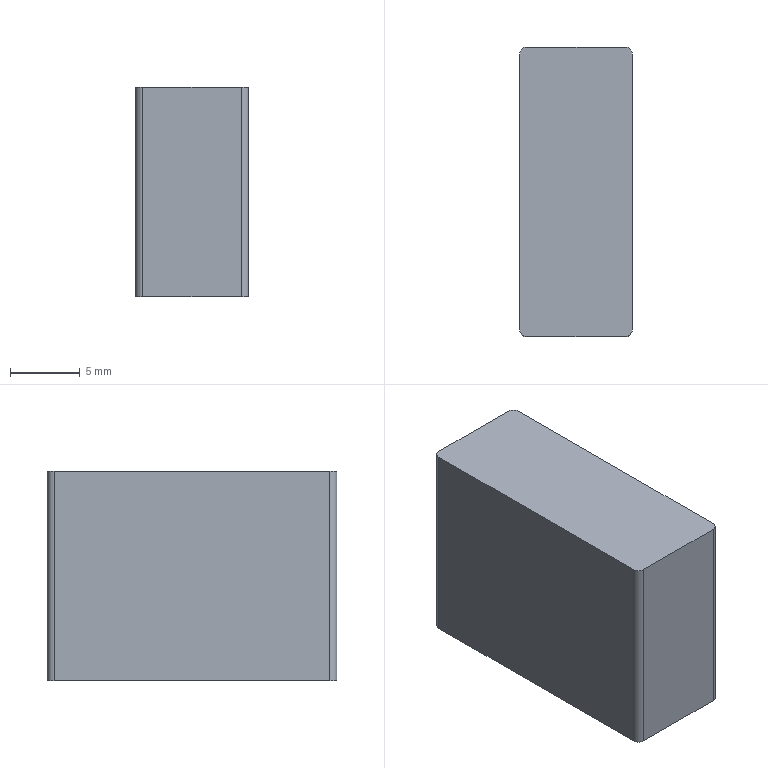Part | NX | features BREP 1 | 1 solid | 10 faces | box 8.05 x 20.702 x 15 mm | volume 2497 mm3 | plane 6 | cylinder 4 | commonest cylinder face diameters 1 x4
STEP:
#1=CARTESIAN_POINT('',(-3.525,10.351,-25.6));
#2=VERTEX_POINT('',#1);
#3=CARTESIAN_POINT('',(-4.025,9.851,-25.6));
#4=VERTEX_POINT('',#3);
#5=CARTESIAN_POINT('',(-3.525,9.851,-25.6));
#6=DIRECTION('',(0.,0.,1.));
#7=DIRECTION('',(1.,0.,0.));
#8=AXIS2_PLACEMENT_3D('',#5,#6,#7);
#9=CIRCLE('',#8,0.5);
#10=EDGE_CURVE('',#2,#4,#9,.T.);
#11=ORIENTED_EDGE('',*,*,#10,.F.);
#12=CARTESIAN_POINT('',(-3.525,10.351,-40.6));
#13=VERTEX_POINT('',#12);
#14=CARTESIAN_POINT('',(-3.525,10.351,-40.6));
#15=DIRECTION('',(0.,0.,1.));
#16=VECTOR('',#15,1000.);
#17=LINE('',#14,#16);
#18=EDGE_CURVE('',#13,#2,#17,.T.);
#19=ORIENTED_EDGE('',*,*,#18,.F.);
#20=CARTESIAN_POINT('',(-4.025,9.851,-40.6));
#21=VERTEX_POINT('',#20);
#22=CARTESIAN_POINT('',(-3.525,9.851,-40.6));
#23=DIRECTION('',(0.,0.,1.));
#24=DIRECTION('',(1.,0.,0.));
#25=AXIS2_PLACEMENT_3D('',#22,#23,#24);
#26=CIRCLE('',#25,0.5);
#27=EDGE_CURVE('',#13,#21,#26,.T.);
#28=ORIENTED_EDGE('',*,*,#27,.T.);
#29=CARTESIAN_POINT('',(-4.025,9.851,-40.6));
#30=DIRECTION('',(0.,0.,1.));
#31=VECTOR('',#30,1000.);
#32=LINE('',#29,#31);
#33=EDGE_CURVE('',#21,#4,#32,.T.);
#34=ORIENTED_EDGE('',*,*,#33,.T.);
#35=EDGE_LOOP('',(#11,#19,#28,#34));
#36=FACE_BOUND('',#35,.T.);
#37=CARTESIAN_POINT('',(-3.525,9.851,-40.6));
#38=DIRECTION('',(0.,0.,1.));
#39=DIRECTION('',(-1.,0.,0.));
#40=AXIS2_PLACEMENT_3D('',#37,#38,#39);
#41=CYLINDRICAL_SURFACE('',#40,0.5);
#42=ADVANCED_FACE('',(#36),#41,.T.);
#43=CARTESIAN_POINT('',(-4.025,-9.851,-25.6));
#44=VERTEX_POINT('',#43);
#45=CARTESIAN_POINT('',(-4.025,-9.851,-25.6));
#46=DIRECTION('',(0.,1.,0.));
#47=VECTOR('',#46,1000.);
#48=LINE('',#45,#47);
#49=EDGE_CURVE('',#44,#4,#48,.T.);
#50=ORIENTED_EDGE('',*,*,#49,.T.);
#51=ORIENTED_EDGE('',*,*,#33,.F.);
#52=CARTESIAN_POINT('',(-4.025,-9.851,-40.6));
#53=VERTEX_POINT('',#52);
#54=CARTESIAN_POINT('',(-4.025,-9.851,-40.6));
#55=DIRECTION('',(0.,1.,0.));
#56=VECTOR('',#55,1000.);
#57=LINE('',#54,#56);
#58=EDGE_CURVE('',#53,#21,#57,.T.);
#59=ORIENTED_EDGE('',*,*,#58,.F.);
#60=CARTESIAN_POINT('',(-4.025,-9.851,-40.6));
#61=DIRECTION('',(0.,0.,1.));
#62=VECTOR('',#61,1000.);
#63=LINE('',#60,#62);
#64=EDGE_CURVE('',#53,#44,#63,.T.);
#65=ORIENTED_EDGE('',*,*,#64,.T.);
#66=EDGE_LOOP('',(#50,#51,#59,#65));
#67=FACE_BOUND('',#66,.T.);
#68=CARTESIAN_POINT('',(-4.025,-9.851,-40.6));
#69=DIRECTION('',(1.,0.,0.));
#70=DIRECTION('',(0.,0.,1.));
#71=AXIS2_PLACEMENT_3D('',#68,#69,#70);
#72=PLANE('',#71);
#73=ADVANCED_FACE('',(#67),#72,.F.);
#74=CARTESIAN_POINT('',(-3.525,-10.351,-25.6));
#75=VERTEX_POINT('',#74);
#76=CARTESIAN_POINT('',(-3.525,-9.851,-25.6));
#77=DIRECTION('',(0.,0.,1.));
#78=DIRECTION('',(1.,0.,0.));
#79=AXIS2_PLACEMENT_3D('',#76,#77,#78);
#80=CIRCLE('',#79,0.5);
#81=EDGE_CURVE('',#44,#75,#80,.T.);
#82=ORIENTED_EDGE('',*,*,#81,.F.);
#83=ORIENTED_EDGE('',*,*,#64,.F.);
#84=CARTESIAN_POINT('',(-3.525,-10.351,-40.6));
#85=VERTEX_POINT('',#84);
#86=CARTESIAN_POINT('',(-3.525,-9.851,-40.6));
#87=DIRECTION('',(0.,0.,1.));
#88=DIRECTION('',(1.,0.,0.));
#89=AXIS2_PLACEMENT_3D('',#86,#87,#88);
#90=CIRCLE('',#89,0.5);
#91=EDGE_CURVE('',#53,#85,#90,.T.);
#92=ORIENTED_EDGE('',*,*,#91,.T.);
#93=CARTESIAN_POINT('',(-3.525,-10.351,-40.6));
#94=DIRECTION('',(0.,0.,1.));
#95=VECTOR('',#94,1000.);
#96=LINE('',#93,#95);
#97=EDGE_CURVE('',#85,#75,#96,.T.);
#98=ORIENTED_EDGE('',*,*,#97,.T.);
#99=EDGE_LOOP('',(#82,#83,#92,#98));
#100=FACE_BOUND('',#99,.T.);
#101=CARTESIAN_POINT('',(-3.525,-9.851,-40.6));
#102=DIRECTION('',(0.,0.,1.));
#103=DIRECTION('',(-1.,0.,0.));
#104=AXIS2_PLACEMENT_3D('',#101,#102,#103);
#105=CYLINDRICAL_SURFACE('',#104,0.5);
#106=ADVANCED_FACE('',(#100),#105,.T.);
#107=CARTESIAN_POINT('',(3.525,-10.351,-25.6));
#108=VERTEX_POINT('',#107);
#109=CARTESIAN_POINT('',(3.525,-10.351,-25.6));
#110=DIRECTION('',(-1.,0.,0.));
#111=VECTOR('',#110,1000.);
#112=LINE('',#109,#111);
#113=EDGE_CURVE('',#108,#75,#112,.T.);
#114=ORIENTED_EDGE('',*,*,#113,.T.);
#115=ORIENTED_EDGE('',*,*,#97,.F.);
#116=CARTESIAN_POINT('',(3.525,-10.351,-40.6));
#117=VERTEX_POINT('',#116);
#118=CARTESIAN_POINT('',(3.525,-10.351,-40.6));
#119=DIRECTION('',(-1.,0.,0.));
#120=VECTOR('',#119,1000.);
#121=LINE('',#118,#120);
#122=EDGE_CURVE('',#117,#85,#121,.T.);
#123=ORIENTED_EDGE('',*,*,#122,.F.);
#124=CARTESIAN_POINT('',(3.525,-10.351,-40.6));
#125=DIRECTION('',(0.,0.,1.));
#126=VECTOR('',#125,1000.);
#127=LINE('',#124,#126);
#128=EDGE_CURVE('',#117,#108,#127,.T.);
#129=ORIENTED_EDGE('',*,*,#128,.T.);
#130=EDGE_LOOP('',(#114,#115,#123,#129));
#131=FACE_BOUND('',#130,.T.);
#132=CARTESIAN_POINT('',(3.525,-10.351,-40.6));
#133=DIRECTION('',(0.,1.,0.));
#134=DIRECTION('',(0.,0.,-1.));
#135=AXIS2_PLACEMENT_3D('',#132,#133,#134);
#136=PLANE('',#135);
#137=ADVANCED_FACE('',(#131),#136,.F.);
#138=CARTESIAN_POINT('',(4.025,-9.851,-25.6));
#139=VERTEX_POINT('',#138);
#140=CARTESIAN_POINT('',(3.525,-9.851,-25.6));
#141=DIRECTION('',(0.,0.,1.));
#142=DIRECTION('',(1.,0.,0.));
#143=AXIS2_PLACEMENT_3D('',#140,#141,#142);
#144=CIRCLE('',#143,0.5);
#145=EDGE_CURVE('',#108,#139,#144,.T.);
#146=ORIENTED_EDGE('',*,*,#145,.F.);
#147=ORIENTED_EDGE('',*,*,#128,.F.);
#148=CARTESIAN_POINT('',(4.025,-9.851,-40.6));
#149=VERTEX_POINT('',#148);
#150=CARTESIAN_POINT('',(3.525,-9.851,-40.6));
#151=DIRECTION('',(0.,0.,1.));
#152=DIRECTION('',(1.,0.,0.));
#153=AXIS2_PLACEMENT_3D('',#150,#151,#152);
#154=CIRCLE('',#153,0.5);
#155=EDGE_CURVE('',#117,#149,#154,.T.);
#156=ORIENTED_EDGE('',*,*,#155,.T.);
#157=CARTESIAN_POINT('',(4.025,-9.851,-40.6));
#158=DIRECTION('',(0.,0.,1.));
#159=VECTOR('',#158,1000.);
#160=LINE('',#157,#159);
#161=EDGE_CURVE('',#149,#139,#160,.T.);
#162=ORIENTED_EDGE('',*,*,#161,.T.);
#163=EDGE_LOOP('',(#146,#147,#156,#162));
#164=FACE_BOUND('',#163,.T.);
#165=CARTESIAN_POINT('',(3.525,-9.851,-40.6));
#166=DIRECTION('',(0.,0.,1.));
#167=DIRECTION('',(-1.,0.,0.));
#168=AXIS2_PLACEMENT_3D('',#165,#166,#167);
#169=CYLINDRICAL_SURFACE('',#168,0.5);
#170=ADVANCED_FACE('',(#164),#169,.T.);
#171=CARTESIAN_POINT('',(4.025,9.851,-25.6));
#172=VERTEX_POINT('',#171);
#173=CARTESIAN_POINT('',(4.025,9.851,-25.6));
#174=DIRECTION('',(0.,-1.,0.));
#175=VECTOR('',#174,1000.);
#176=LINE('',#173,#175);
#177=EDGE_CURVE('',#172,#139,#176,.T.);
#178=ORIENTED_EDGE('',*,*,#177,.T.);
#179=ORIENTED_EDGE('',*,*,#161,.F.);
#180=CARTESIAN_POINT('',(4.025,9.851,-40.6));
#181=VERTEX_POINT('',#180);
#182=CARTESIAN_POINT('',(4.025,9.851,-40.6));
#183=DIRECTION('',(0.,-1.,0.));
#184=VECTOR('',#183,1000.);
#185=LINE('',#182,#184);
#186=EDGE_CURVE('',#181,#149,#185,.T.);
#187=ORIENTED_EDGE('',*,*,#186,.F.);
#188=CARTESIAN_POINT('',(4.025,9.851,-40.6));
#189=DIRECTION('',(0.,0.,1.));
#190=VECTOR('',#189,1000.);
#191=LINE('',#188,#190);
#192=EDGE_CURVE('',#181,#172,#191,.T.);
#193=ORIENTED_EDGE('',*,*,#192,.T.);
#194=EDGE_LOOP('',(#178,#179,#187,#193));
#195=FACE_BOUND('',#194,.T.);
#196=CARTESIAN_POINT('',(4.025,9.851,-40.6));
#197=DIRECTION('',(-1.,0.,0.));
#198=DIRECTION('',(0.,1.,0.));
#199=AXIS2_PLACEMENT_3D('',#196,#197,#198);
#200=PLANE('',#199);
#201=ADVANCED_FACE('',(#195),#200,.F.);
#202=CARTESIAN_POINT('',(3.525,10.351,-25.6));
#203=VERTEX_POINT('',#202);
#204=CARTESIAN_POINT('',(3.525,9.851,-25.6));
#205=DIRECTION('',(0.,0.,1.));
#206=DIRECTION('',(1.,0.,0.));
#207=AXIS2_PLACEMENT_3D('',#204,#205,#206);
#208=CIRCLE('',#207,0.5);
#209=EDGE_CURVE('',#172,#203,#208,.T.);
#210=ORIENTED_EDGE('',*,*,#209,.F.);
#211=ORIENTED_EDGE('',*,*,#192,.F.);
#212=CARTESIAN_POINT('',(3.525,10.351,-40.6));
#213=VERTEX_POINT('',#212);
#214=CARTESIAN_POINT('',(3.525,9.851,-40.6));
#215=DIRECTION('',(0.,0.,1.));
#216=DIRECTION('',(1.,0.,0.));
#217=AXIS2_PLACEMENT_3D('',#214,#215,#216);
#218=CIRCLE('',#217,0.5);
#219=EDGE_CURVE('',#181,#213,#218,.T.);
#220=ORIENTED_EDGE('',*,*,#219,.T.);
#221=CARTESIAN_POINT('',(3.525,10.351,-40.6));
#222=DIRECTION('',(0.,0.,1.));
#223=VECTOR('',#222,1000.);
#224=LINE('',#221,#223);
#225=EDGE_CURVE('',#213,#203,#224,.T.);
#226=ORIENTED_EDGE('',*,*,#225,.T.);
#227=EDGE_LOOP('',(#210,#211,#220,#226));
#228=FACE_BOUND('',#227,.T.);
#229=CARTESIAN_POINT('',(3.525,9.851,-40.6));
#230=DIRECTION('',(0.,0.,1.));
#231=DIRECTION('',(-1.,0.,0.));
#232=AXIS2_PLACEMENT_3D('',#229,#230,#231);
#233=CYLINDRICAL_SURFACE('',#232,0.5);
#234=ADVANCED_FACE('',(#228),#233,.T.);
#235=CARTESIAN_POINT('',(-3.525,10.351,-25.6));
#236=DIRECTION('',(1.,0.,0.));
#237=VECTOR('',#236,1000.);
#238=LINE('',#235,#237);
#239=EDGE_CURVE('',#2,#203,#238,.T.);
#240=ORIENTED_EDGE('',*,*,#239,.T.);
#241=ORIENTED_EDGE('',*,*,#225,.F.);
#242=CARTESIAN_POINT('',(-3.525,10.351,-40.6));
#243=DIRECTION('',(1.,0.,0.));
#244=VECTOR('',#243,1000.);
#245=LINE('',#242,#244);
#246=EDGE_CURVE('',#13,#213,#245,.T.);
#247=ORIENTED_EDGE('',*,*,#246,.F.);
#248=ORIENTED_EDGE('',*,*,#18,.T.);
#249=EDGE_LOOP('',(#240,#241,#247,#248));
#250=FACE_BOUND('',#249,.T.);
#251=CARTESIAN_POINT('',(-3.525,10.351,-40.6));
#252=DIRECTION('',(0.,-1.,0.));
#253=DIRECTION('',(0.,0.,1.));
#254=AXIS2_PLACEMENT_3D('',#251,#252,#253);
#255=PLANE('',#254);
#256=ADVANCED_FACE('',(#250),#255,.F.);
#257=ORIENTED_EDGE('',*,*,#27,.F.);
#258=ORIENTED_EDGE('',*,*,#246,.T.);
#259=ORIENTED_EDGE('',*,*,#219,.F.);
#260=ORIENTED_EDGE('',*,*,#186,.T.);
#261=ORIENTED_EDGE('',*,*,#155,.F.);
#262=ORIENTED_EDGE('',*,*,#122,.T.);
#263=ORIENTED_EDGE('',*,*,#91,.F.);
#264=ORIENTED_EDGE('',*,*,#58,.T.);
#265=EDGE_LOOP('',(#257,#258,#259,#260,#261,#262,#263,#264));
#266=FACE_BOUND('',#265,.T.);
#267=CARTESIAN_POINT('',(-3.525,9.851,-40.6));
#268=DIRECTION('',(0.,0.,1.));
#269=DIRECTION('',(-1.,0.,0.));
#270=AXIS2_PLACEMENT_3D('',#267,#268,#269);
#271=PLANE('',#270);
#272=ADVANCED_FACE('',(#266),#271,.F.);
#273=ORIENTED_EDGE('',*,*,#10,.T.);
#274=ORIENTED_EDGE('',*,*,#49,.F.);
#275=ORIENTED_EDGE('',*,*,#81,.T.);
#276=ORIENTED_EDGE('',*,*,#113,.F.);
#277=ORIENTED_EDGE('',*,*,#145,.T.);
#278=ORIENTED_EDGE('',*,*,#177,.F.);
#279=ORIENTED_EDGE('',*,*,#209,.T.);
#280=ORIENTED_EDGE('',*,*,#239,.F.);
#281=EDGE_LOOP('',(#273,#274,#275,#276,#277,#278,#279,#280));
#282=FACE_BOUND('',#281,.T.);
#283=CARTESIAN_POINT('',(-3.525,9.851,-25.6));
#284=DIRECTION('',(0.,0.,1.));
#285=DIRECTION('',(-1.,0.,0.));
#286=AXIS2_PLACEMENT_3D('',#283,#284,#285);
#287=PLANE('',#286);
#288=ADVANCED_FACE('',(#282),#287,.T.);
#289=CLOSED_SHELL('',(#42,#73,#106,#137,#170,#201,#234,#256,#272,#288));
#290=MANIFOLD_SOLID_BREP('',#289);
#291=(LENGTH_UNIT()NAMED_UNIT(*)SI_UNIT(.MILLI.,.METRE.));
#292=UNCERTAINTY_MEASURE_WITH_UNIT(LENGTH_MEASURE(0.00001),#291,'','');
#293=(NAMED_UNIT(*)PLANE_ANGLE_UNIT()SI_UNIT($,.RADIAN.));
#294=(NAMED_UNIT(*)SI_UNIT($,.STERADIAN.)SOLID_ANGLE_UNIT());
#295=(GEOMETRIC_REPRESENTATION_CONTEXT(3)GLOBAL_UNCERTAINTY_ASSIGNED_CONTEXT((#292))GLOBAL_UNIT_ASSIGNED_CONTEXT((#291,#293,#294))REPRESENTATION_CONTEXT('',''));
#296=ADVANCED_BREP_SHAPE_REPRESENTATION('',(#290),#295);